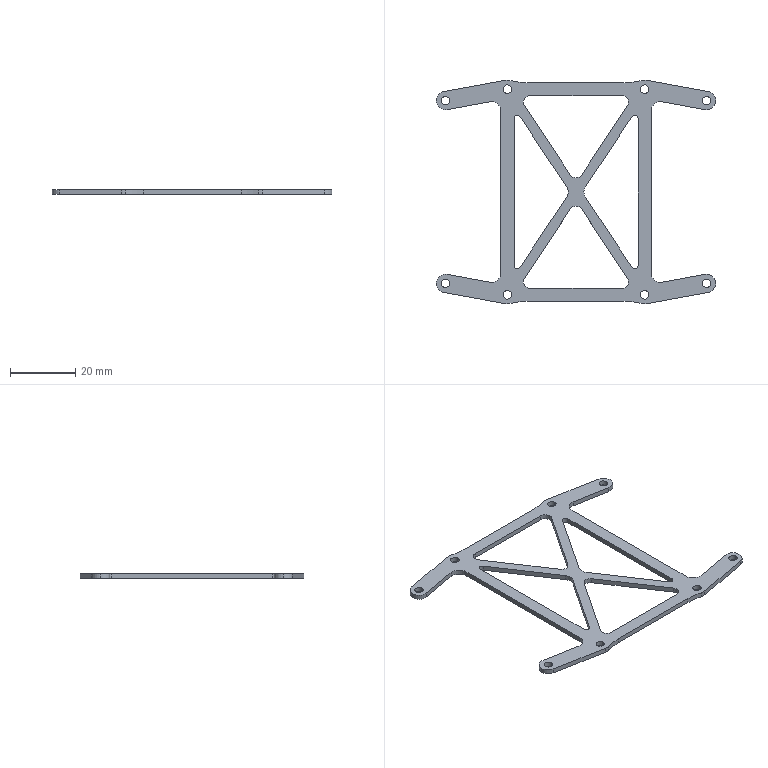Part | SolidWorks | features Fillet 4, Extrusion 1 | 1 solid | 75 faces | box 85.6 x 68.6 x 1.5 mm | volume 2523 mm3 | cylinder 49 | plane 26 | commonest cylinder face diameters 2.6 x16 5.6 x10 4 x8 6 x7 2 x4 40 x4